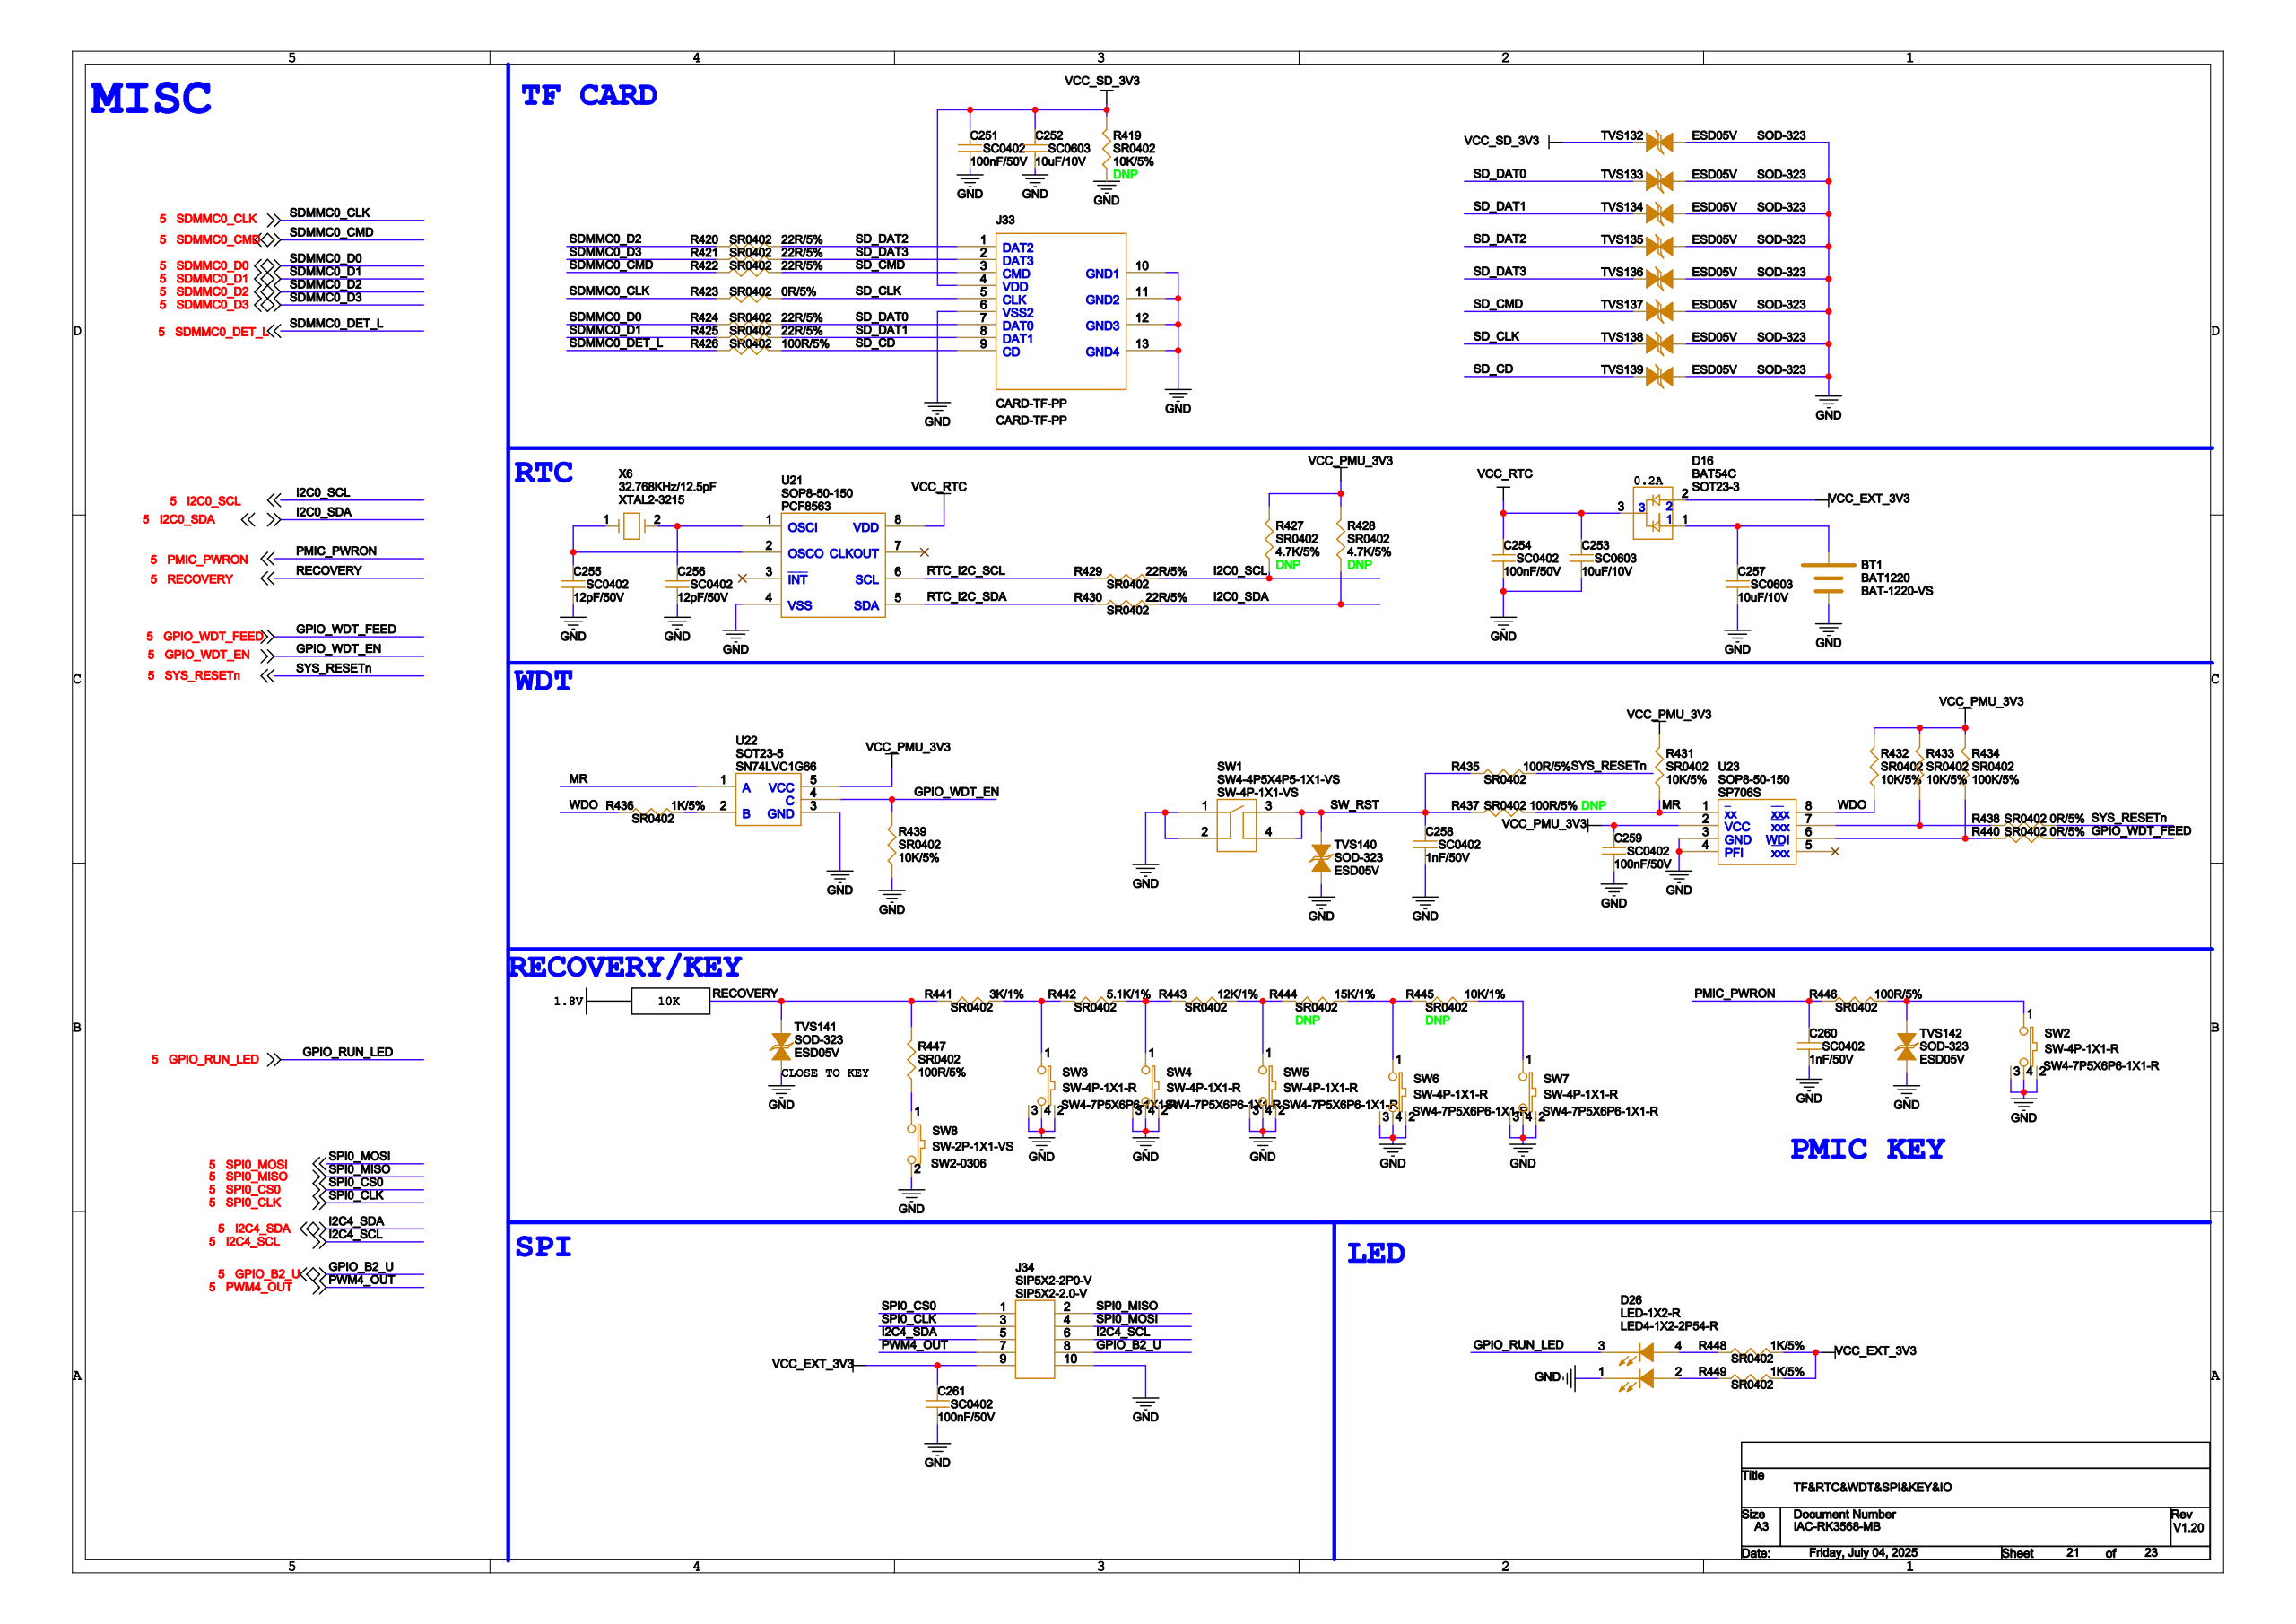Circuit board | Cadence Allegro | 1138 parts | 722 nets | one sheet of the schematic
Parts on this sheet (reference | value | footprint):
BT1 | BAT1220 | BAT-1220-VS
C251 | 100nF/50V | SC0402
C252 | 10uF/10V | SC0603
C253 | 10uF/10V | SC0603
C254 | 100nF/50V | SC0402
C255 | 12pF/50V | SC0402
C256 | 12pF/50V | SC0402
C257 | 10uF/10V | SC0603
C258 | 1nF/50V | SC0402
C259 | 100nF/50V | SC0402
C260 | 1nF/50V | SC0402
C261 | 100nF/50V | SC0402
D16 | BAT54C | SOT23-3
D26 | LED-1X2-R | LED4-1X2-2P54-R
J33 | CARD-TF-PP | CARD-TF-PP
J34 | SIP5X2-2.0-V | SIP5X2-2P0-V
R419 | 10K/5% | SR0402
R420 | 22R/5% | SR0402
R421 | 22R/5% | SR0402
R422 | 22R/5% | SR0402
R423 | 0R/5% | SR0402
R424 | 22R/5% | SR0402
R425 | 22R/5% | SR0402
R426 | 100R/5% | SR0402
R427 | 4.7K/5% | SR0402
R428 | 4.7K/5% | SR0402
R429 | 22R/5% | SR0402
R430 | 22R/5% | SR0402
R431 | 10K/5% | SR0402
R432 | 10K/5% | SR0402
R433 | 10K/5% | SR0402
R434 | 100K/5% | SR0402
R435 | 100R/5% | SR0402
R436 | 1K/5% | SR0402
R437 | 100R/5% | SR0402
R438 | 0R/5% | SR0402
R439 | 10K/5% | SR0402
R440 | 0R/5% | SR0402
R441 | 3K/1% | SR0402
R442 | 5.1K/1% | SR0402
R443 | 12K/1% | SR0402
R444 | 15K/1% | SR0402
R445 | 10K/1% | SR0402
R446 | 100R/5% | SR0402
R447 | 100R/5% | SR0402
R448 | 1K/5% | SR0402
R449 | 1K/5% | SR0402
SW1 | SW-4P-1X1-VS | SW4-4P5X4P5-1X1-VS
SW2 | SW-4P-1X1-R | SW4-7P5X6P6-1X1-R
SW3 | SW-4P-1X1-R | SW4-7P5X6P6-1X1-R
SW4 | SW-4P-1X1-R | SW4-7P5X6P6-1X1-R
SW5 | SW-4P-1X1-R | SW4-7P5X6P6-1X1-R
SW6 | SW-4P-1X1-R | SW4-7P5X6P6-1X1-R
SW7 | SW-4P-1X1-R | SW4-7P5X6P6-1X1-R
SW8 | SW-2P-1X1-VS | SW2-0306
TVS132 | ESD05V | SOD-323
TVS133 | ESD05V | SOD-323
TVS134 | ESD05V | SOD-323
TVS135 | ESD05V | SOD-323
TVS136 | ESD05V | SOD-323
TVS137 | ESD05V | SOD-323
TVS138 | ESD05V | SOD-323
TVS139 | ESD05V | SOD-323
TVS140 | ESD05V | SOD-323
TVS141 | ESD05V | SOD-323
TVS142 | ESD05V | SOD-323
U21 | PCF8563 | SOP8-50-150
U22 | SN74LVC1G66 | SOT23-5
U23 | SP706S | SOP8-50-150
X6 | 32.768KHz/12.5pF | XTAL2-3215
Nets of these parts (net: part-pin ...):
N19611831: BT1-1 C257-1 D16-1
VCC_EXT_3V3: C261-1 D16-2 J34-9 R448-1 R449-1
VCC_RTC: C253-1 C254-1 D16-3 U21-8
GND: BT1-2 C251-2 C252-2 C253-2 C254-2 C255-2 C256-2 C257-2 C258-2 C259-2 C260-2 C261-2 D26-1 J33-6 J33-10 J33-11 J33-12 J33-13 J34-10 R419-1 R439-1 SW1-1 SW1-2 SW2-2 SW2-3 SW2-4 SW3-2 SW3-3 SW3-4 SW4-2 SW4-3 SW4-4 SW5-2 SW5-3 SW5-4 SW6-2 SW6-3 SW6-4 SW7-2 SW7-3 SW7-4 SW8-2 TVS132-2 TVS133-2 TVS134-2 TVS135-2 TVS136-2 TVS137-2 TVS138-2 TVS139-2 TVS140-1 TVS141-1 TVS142-1 U21-4 U22-3 U23-3 U23-4
VCC_SD_3V3: C251-1 C252-1 J33-4 R419-2 TVS132-1
SD_DAT0: J33-7 R424-2 TVS133-1
SD_DAT1: J33-8 R425-2 TVS134-1
SD_DAT2: J33-1 R420-2 TVS135-1
SD_DAT3: J33-2 R421-2 TVS136-1
SD_CMD: J33-3 R422-2 TVS137-1
SD_CLK: J33-5 R423-2 TVS138-1
SD_CD: J33-9 R426-2 TVS139-1
SW_RST: C258-1 R435-1 R437-1 SW1-3 SW1-4 TVS140-2
RECOVERY: R441-2 R447-2 TVS141-2
N4106854: R446-2 SW2-1 TVS142-2
N4101528: R441-1 R442-2 SW3-1
N4102261: R442-1 R443-2 SW4-1
N4102618: R443-1 R444-2 SW5-1
N4106012: R444-1 R445-2 SW6-1
N4106234: R445-1 SW7-1
PMIC_PWRON: C260-1 R446-1
N5182501: D26-2 R449-2
N5182511: D26-4 R448-2
GPIO_RUN_LED: D26-3
SPI0_CS0: J34-1
SPI0_MISO: J34-2
SPI0_CLK: J34-3
SPI0_MOSI: J34-4
I2C4_SDA: J34-5
I2C4_SCL: J34-6
PWM4_OUT: J34-7
GPIO_B2_U: J34-8
N19646478: R434-1 R440-1 U23-6
VCC_PMU_3V3: C259-1 R427-2 R428-2 R431-2 R432-2 R433-2 R434-2 U22-5 U23-2
SDMMC0_DET_L: R426-1
SYS_RESETN: R435-2 R438-2
MR: R431-1 R437-2 U22-1 U23-1
N4103569: R447-1 SW8-1
GPIO_WDT_EN: R439-2 U22-4
GPIO_WDT_FEED: R440-2
I2C0_SCL: R427-1 R429-2
I2C0_SDA: R428-1 R430-2
SDMMC0_CLK: R423-1
SDMMC0_CMD: R422-1
SDMMC0_D0: R424-1
SDMMC0_D1: R425-1
SDMMC0_D2: R420-1
SDMMC0_D3: R421-1
N6504164: C256-1 U21-1 X6-2
N19611886: C255-1 U21-2 X6-1
RTC_I2C_SCL: R429-1 U21-6
RTC_I2C_SDA: R430-1 U21-5
N4093138: R436-2 U22-2
N19646487: R433-1 R438-1 U23-7
WDO: R432-1 R436-1 U23-8